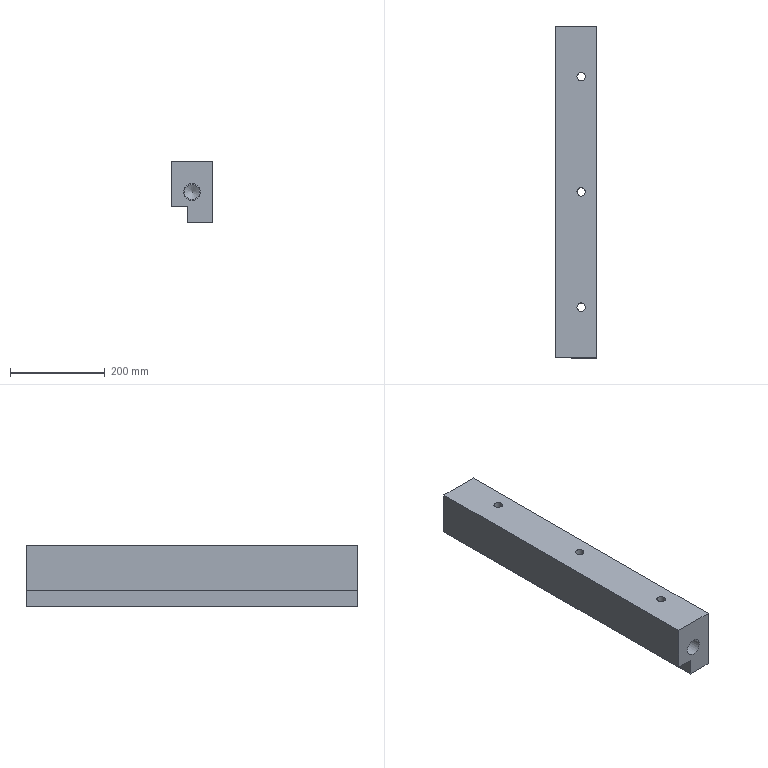Part | STEP file | CC01 | 1 solid | 23 faces | box 88 x 700 x 130 mm | volume 6902512 mm3 | plane 10 | cylinder 9 | cone 4 | commonest cylinder face diameters 18 x3 12 x2 31.8 x2 36 x2